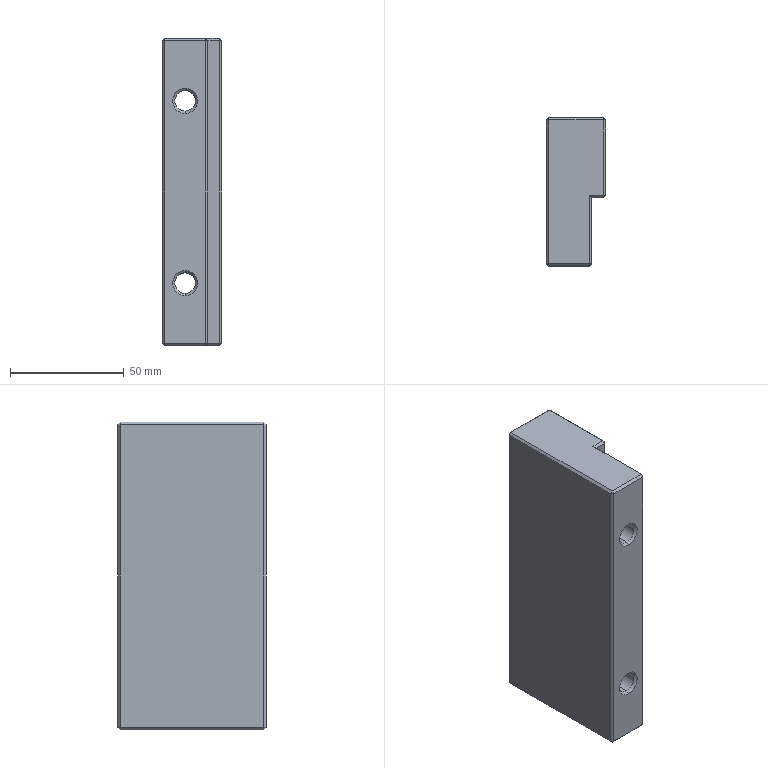Part | STEP file | Trilho - Torre - 1 cav - 5 | 1 solid | 53 faces | box 26 x 65 x 135 mm | volume 189332 mm3 | plane 37 | cone 8 | cylinder 8 | commonest cylinder face diameters 9 x4 15 x4